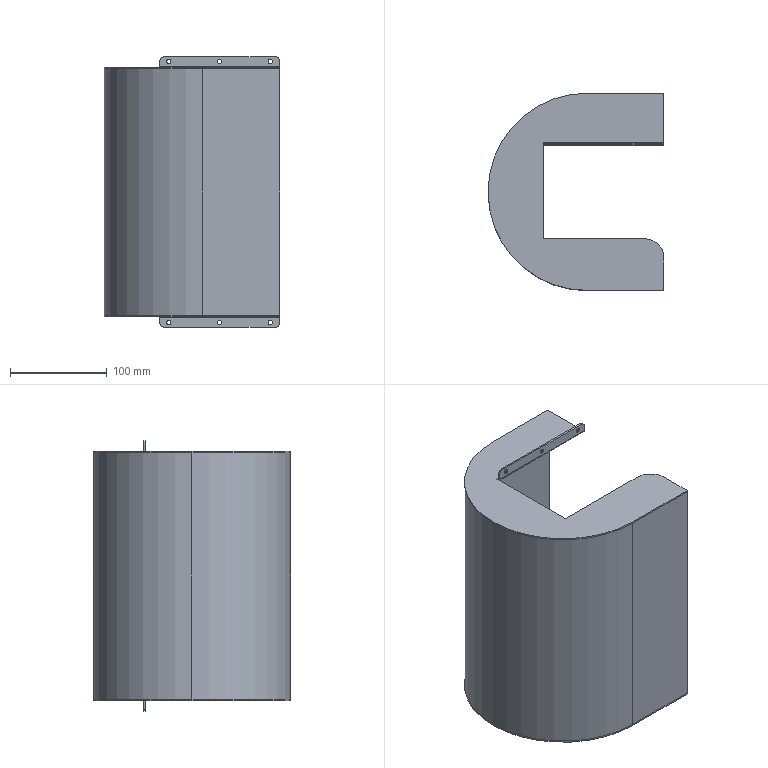Part | SolidWorks | features FlatPattern 3, SMBaseFlange 2, SheetMetal 2, 3DProfileFeature 1, EdgeFlange 1, Fillet 1, HoleWzd 1, MirrorSolid 1 | 3 solids | 76 faces | box 182 x 204 x 280 mm | volume 308459 mm3 | plane 46 | cylinder 30 | commonest cylinder face diameters 4.5 x12 204 x6 10 x4 1.473 x2 4.473 x2 40 x2